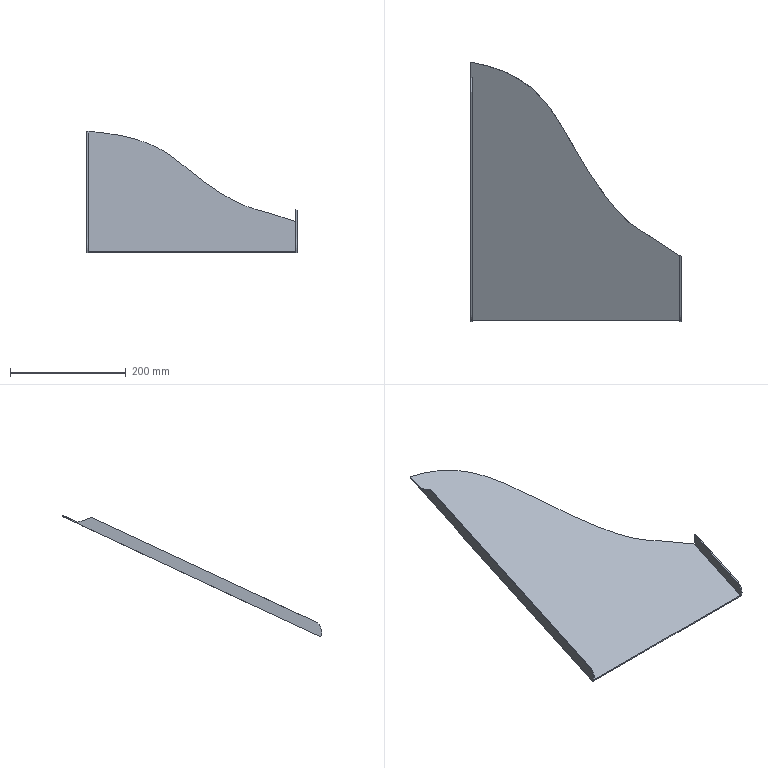Part | NX | features solid 2 | 1 solid | 13 faces | box 363.564 x 448.767 x 210.596 mm | volume 253893 mm3 | plane 10 | cylinder 2 | spline 1 | commonest cylinder face diameters 40 x2
STEP:
#1=CARTESIAN_POINT('',(111.564,-680.,-297.684));
#2=VERTEX_POINT('',#1);
#3=CARTESIAN_POINT('',(-248.,-680.,-297.684));
#4=VERTEX_POINT('',#3);
#5=CARTESIAN_POINT('',(188.564,-680.,-297.684));
#6=DIRECTION('',(1.,0.,0.));
#7=VECTOR('',#6,1000.);
#8=LINE('',#5,#7);
#9=EDGE_CURVE('',#2,#4,#8,.F.);
#10=ORIENTED_EDGE('',*,*,#9,.T.);
#11=CARTESIAN_POINT('',(-248.,-680.,-299.891));
#12=VERTEX_POINT('',#11);
#13=CARTESIAN_POINT('',(-248.,-680.,-430.));
#14=DIRECTION('',(0.,0.,1.));
#15=VECTOR('',#14,1000.);
#16=LINE('',#13,#15);
#17=EDGE_CURVE('',#4,#12,#16,.F.);
#18=ORIENTED_EDGE('',*,*,#17,.T.);
#19=CARTESIAN_POINT('',(111.564,-680.,-299.891));
#20=VERTEX_POINT('',#19);
#21=CARTESIAN_POINT('',(188.564,-680.,-299.891));
#22=DIRECTION('',(1.,0.,0.));
#23=VECTOR('',#22,1000.);
#24=LINE('',#21,#23);
#25=EDGE_CURVE('',#20,#12,#24,.F.);
#26=ORIENTED_EDGE('',*,*,#25,.F.);
#27=CARTESIAN_POINT('',(111.564,-680.,-430.));
#28=DIRECTION('',(0.,0.,1.));
#29=VECTOR('',#28,1000.);
#30=LINE('',#27,#29);
#31=EDGE_CURVE('',#2,#20,#30,.F.);
#32=ORIENTED_EDGE('',*,*,#31,.F.);
#33=EDGE_LOOP('',(#10,#18,#26,#32));
#34=FACE_BOUND('',#33,.T.);
#35=CARTESIAN_POINT('',(188.564,-680.,-430.));
#36=DIRECTION('',(0.,1.,0.));
#37=DIRECTION('',(-1.,0.,0.));
#38=AXIS2_PLACEMENT_3D('',#35,#36,#37);
#39=PLANE('',#38);
#40=ADVANCED_FACE('',(#34),#39,.F.);
#41=CARTESIAN_POINT('',(111.564,-567.729,-245.332));
#42=VERTEX_POINT('',#41);
#43=CARTESIAN_POINT('',(111.564,-570.845,-246.785));
#44=DIRECTION('',(0.,-0.9063,-0.4226));
#45=VECTOR('',#44,1000.);
#46=LINE('',#43,#45);
#47=EDGE_CURVE('',#42,#2,#46,.T.);
#48=ORIENTED_EDGE('',*,*,#47,.F.);
#49=CARTESIAN_POINT('',(-250.,-233.107,-89.295));
#50=VERTEX_POINT('',#49);
#51=CARTESIAN_POINT('',(111.564,-567.729,-245.332));
#52=CARTESIAN_POINT('',(102.698,-561.923,-242.624));
#53=CARTESIAN_POINT('',(89.392,-553.224,-238.568));
#54=CARTESIAN_POINT('',(71.68,-541.588,-233.142));
#55=CARTESIAN_POINT('',(58.379,-532.881,-229.082));
#56=CARTESIAN_POINT('',(44.434,-524.954,-225.385));
#57=CARTESIAN_POINT('',(26.687,-513.356,-219.977));
#58=CARTESIAN_POINT('',(11.101,-499.177,-213.365));
#59=CARTESIAN_POINT('',(-3.01,-483.135,-205.885));
#60=CARTESIAN_POINT('',(-16.196,-466.641,-198.194));
#61=CARTESIAN_POINT('',(-31.486,-445.373,-188.276));
#62=CARTESIAN_POINT('',(-48.725,-419.266,-176.102));
#63=CARTESIAN_POINT('',(-64.763,-392.515,-163.628));
#64=CARTESIAN_POINT('',(-80.04,-365.364,-150.967));
#65=CARTESIAN_POINT('',(-95.517,-338.302,-138.348));
#66=CARTESIAN_POINT('',(-112.708,-312.215,-126.184));
#67=CARTESIAN_POINT('',(-129.476,-292.193,-116.847));
#68=CARTESIAN_POINT('',(-145.224,-277.575,-110.031));
#69=CARTESIAN_POINT('',(-157.985,-267.745,-105.447));
#70=CARTESIAN_POINT('',(-171.635,-259.126,-101.428));
#71=CARTESIAN_POINT('',(-186.187,-251.702,-97.966));
#72=CARTESIAN_POINT('',(-201.622,-245.418,-95.036));
#73=CARTESIAN_POINT('',(-222.673,-238.648,-91.879));
#74=CARTESIAN_POINT('',(-238.985,-235.068,-90.209));
#75=CARTESIAN_POINT('',(-250.,-233.107,-89.295));
#76=B_SPLINE_CURVE_WITH_KNOTS('',3,(#51,#52,#53,#54,#55,#56,#57,#58,#59,#60,#61,#62,#63,#64,#65,#66,#67,#68,#69,#70,#71,#72,#73,#74,#75),.UNSPECIFIED.,.F.,.F.,(4,1,1,1,1,1,1,1,1,1,1,1,1,1,1,1,1,1,1,1,1,1,4),(3.45,3.483,3.499,3.516,3.532,3.549,3.581,3.598,3.614,3.647,3.68,3.713,3.745,3.778,3.811,3.844,3.86,3.877,3.893,3.91,3.926,3.942,3.975),.UNSPECIFIED.);
#77=EDGE_CURVE('',#42,#50,#76,.T.);
#78=ORIENTED_EDGE('',*,*,#77,.T.);
#79=CARTESIAN_POINT('',(-250.,-259.971,-101.822));
#80=VERTEX_POINT('',#79);
#81=CARTESIAN_POINT('',(-250.,-570.845,-246.785));
#82=DIRECTION('',(0.,0.9063,0.4226));
#83=VECTOR('',#82,1000.);
#84=LINE('',#81,#83);
#85=EDGE_CURVE('',#50,#80,#84,.F.);
#86=ORIENTED_EDGE('',*,*,#85,.T.);
#87=CARTESIAN_POINT('',(-248.,-259.971,-101.822));
#88=VERTEX_POINT('',#87);
#89=CARTESIAN_POINT('',(-800.,-259.971,-101.822));
#90=DIRECTION('',(1.,0.,0.));
#91=VECTOR('',#90,1000.);
#92=LINE('',#89,#91);
#93=EDGE_CURVE('',#88,#80,#92,.F.);
#94=ORIENTED_EDGE('',*,*,#93,.F.);
#95=CARTESIAN_POINT('',(-248.,-570.845,-246.785));
#96=DIRECTION('',(0.,-0.9063,-0.4226));
#97=VECTOR('',#96,1000.);
#98=LINE('',#95,#97);
#99=EDGE_CURVE('',#88,#4,#98,.T.);
#100=ORIENTED_EDGE('',*,*,#99,.T.);
#101=ORIENTED_EDGE('',*,*,#9,.F.);
#102=EDGE_LOOP('',(#48,#78,#86,#94,#100,#101));
#103=FACE_BOUND('',#102,.T.);
#104=CARTESIAN_POINT('',(-800.,-570.845,-246.785));
#105=DIRECTION('',(0.,-0.4226,0.9063));
#106=DIRECTION('',(0.,-0.9063,-0.4226));
#107=AXIS2_PLACEMENT_3D('',#104,#105,#106);
#108=PLANE('',#107);
#109=ADVANCED_FACE('',(#103),#108,.T.);
#110=ORIENTED_EDGE('',*,*,#77,.F.);
#111=CARTESIAN_POINT('',(111.564,-567.729,-225.471));
#112=VERTEX_POINT('',#111);
#113=CARTESIAN_POINT('',(111.564,-567.729,-267.464));
#114=DIRECTION('',(0.,0.,1.));
#115=VECTOR('',#114,1000.);
#116=LINE('',#113,#115);
#117=EDGE_CURVE('',#42,#112,#116,.T.);
#118=ORIENTED_EDGE('',*,*,#117,.T.);
#119=CARTESIAN_POINT('',(113.564,-569.039,-226.082));
#120=VERTEX_POINT('',#119);
#121=CARTESIAN_POINT('',(111.564,-567.729,-225.471));
#122=CARTESIAN_POINT('',(112.231,-568.166,-225.674));
#123=CARTESIAN_POINT('',(112.898,-568.602,-225.878));
#124=CARTESIAN_POINT('',(113.564,-569.039,-226.082));
#125=B_SPLINE_CURVE_WITH_KNOTS('',3,(#121,#122,#123,#124),.UNSPECIFIED.,.F.,.F.,(4,4),(-0.1295,-0.1271),.UNSPECIFIED.);
#126=EDGE_CURVE('',#112,#120,#125,.T.);
#127=ORIENTED_EDGE('',*,*,#126,.T.);
#128=CARTESIAN_POINT('',(113.564,-569.039,-248.149));
#129=VERTEX_POINT('',#128);
#130=CARTESIAN_POINT('',(113.564,-569.039,-269.178));
#131=DIRECTION('',(0.,0.,1.));
#132=VECTOR('',#131,1000.);
#133=LINE('',#130,#132);
#134=EDGE_CURVE('',#120,#129,#133,.F.);
#135=ORIENTED_EDGE('',*,*,#134,.T.);
#136=CARTESIAN_POINT('',(-250.,-233.107,-91.502));
#137=VERTEX_POINT('',#136);
#138=CARTESIAN_POINT('',(113.564,-569.039,-248.149));
#139=CARTESIAN_POINT('',(104.432,-563.058,-245.36));
#140=CARTESIAN_POINT('',(90.729,-554.091,-241.179));
#141=CARTESIAN_POINT('',(72.473,-542.122,-235.598));
#142=CARTESIAN_POINT('',(58.806,-533.125,-231.402));
#143=CARTESIAN_POINT('',(44.256,-524.862,-227.549));
#144=CARTESIAN_POINT('',(26.021,-512.876,-221.96));
#145=CARTESIAN_POINT('',(6.706,-495.001,-213.625));
#146=CARTESIAN_POINT('',(-13.173,-470.808,-202.344));
#147=CARTESIAN_POINT('',(-31.517,-445.34,-190.467));
#148=CARTESIAN_POINT('',(-48.868,-419.045,-178.206));
#149=CARTESIAN_POINT('',(-65.147,-391.859,-165.529));
#150=CARTESIAN_POINT('',(-80.74,-364.104,-152.586));
#151=CARTESIAN_POINT('',(-96.57,-336.542,-139.734));
#152=CARTESIAN_POINT('',(-114.056,-310.368,-127.529));
#153=CARTESIAN_POINT('',(-134.465,-286.588,-116.44));
#154=CARTESIAN_POINT('',(-158.481,-266.484,-107.065));
#155=CARTESIAN_POINT('',(-187.039,-250.568,-99.644));
#156=CARTESIAN_POINT('',(-217.596,-239.769,-94.608));
#157=CARTESIAN_POINT('',(-239.141,-235.04,-92.403));
#158=CARTESIAN_POINT('',(-250.,-233.107,-91.502));
#159=B_SPLINE_CURVE_WITH_KNOTS('',3,(#138,#139,#140,#141,#142,#143,#144,#145,#146,#147,#148,#149,#150,#151,#152,#153,#154,#155,#156,#157,#158),.UNSPECIFIED.,.F.,.F.,(4,1,1,1,1,1,1,1,1,1,1,1,1,1,1,1,1,1,4),(0.1269,0.16,0.1765,0.1931,0.2097,0.2262,0.2593,0.2924,0.3255,0.3586,0.3918,0.4249,0.458,0.4911,0.5242,0.5573,0.5904,0.6235,0.6566),.UNSPECIFIED.);
#160=EDGE_CURVE('',#129,#137,#159,.T.);
#161=ORIENTED_EDGE('',*,*,#160,.T.);
#162=CARTESIAN_POINT('',(-250.,-233.107,-89.295));
#163=DIRECTION('',(0.,0.,1.));
#164=VECTOR('',#163,1000.);
#165=LINE('',#162,#164);
#166=EDGE_CURVE('',#50,#137,#165,.F.);
#167=ORIENTED_EDGE('',*,*,#166,.F.);
#168=EDGE_LOOP('',(#110,#118,#127,#135,#161,#167));
#169=FACE_BOUND('',#168,.T.);
#170=CARTESIAN_POINT('',(-250.,-233.107,-249.102));
#171=CARTESIAN_POINT('',(-250.,-233.107,-88.342));
#172=CARTESIAN_POINT('',(-239.339,-235.005,-249.102));
#173=CARTESIAN_POINT('',(-239.339,-235.005,-88.342));
#174=CARTESIAN_POINT('',(-218.009,-239.639,-249.102));
#175=CARTESIAN_POINT('',(-218.009,-239.639,-88.342));
#176=CARTESIAN_POINT('',(-186.633,-250.694,-249.102));
#177=CARTESIAN_POINT('',(-186.633,-250.694,-88.342));
#178=CARTESIAN_POINT('',(-157.179,-267.241,-249.102));
#179=CARTESIAN_POINT('',(-157.179,-267.241,-88.342));
#180=CARTESIAN_POINT('',(-131.588,-289.326,-249.102));
#181=CARTESIAN_POINT('',(-131.588,-289.326,-88.342));
#182=CARTESIAN_POINT('',(-110.563,-315.071,-249.102));
#183=CARTESIAN_POINT('',(-110.563,-315.071,-88.342));
#184=CARTESIAN_POINT('',(-92.999,-342.512,-249.102));
#185=CARTESIAN_POINT('',(-92.999,-342.512,-88.342));
#186=CARTESIAN_POINT('',(-77.274,-370.319,-249.102));
#187=CARTESIAN_POINT('',(-77.274,-370.319,-88.342));
#188=CARTESIAN_POINT('',(-61.764,-397.709,-249.102));
#189=CARTESIAN_POINT('',(-61.764,-397.709,-88.342));
#190=CARTESIAN_POINT('',(-45.456,-424.418,-249.102));
#191=CARTESIAN_POINT('',(-45.456,-424.418,-88.342));
#192=CARTESIAN_POINT('',(-28.01,-450.369,-249.102));
#193=CARTESIAN_POINT('',(-28.01,-450.369,-88.342));
#194=CARTESIAN_POINT('',(-12.615,-471.361,-249.102));
#195=CARTESIAN_POINT('',(-12.615,-471.361,-88.342));
#196=CARTESIAN_POINT('',(0.44,-487.186,-249.102));
#197=CARTESIAN_POINT('',(0.44,-487.186,-88.342));
#198=CARTESIAN_POINT('',(10.739,-498.433,-249.102));
#199=CARTESIAN_POINT('',(10.739,-498.433,-88.342));
#200=CARTESIAN_POINT('',(21.663,-508.711,-249.102));
#201=CARTESIAN_POINT('',(21.663,-508.711,-88.342));
#202=CARTESIAN_POINT('',(33.398,-517.826,-249.102));
#203=CARTESIAN_POINT('',(33.398,-517.826,-88.342));
#204=CARTESIAN_POINT('',(43.982,-524.572,-249.102));
#205=CARTESIAN_POINT('',(43.982,-524.572,-88.342));
#206=CARTESIAN_POINT('',(52.969,-529.82,-249.102));
#207=CARTESIAN_POINT('',(52.969,-529.82,-88.342));
#208=CARTESIAN_POINT('',(59.982,-534.012,-249.102));
#209=CARTESIAN_POINT('',(59.982,-534.012,-88.342));
#210=CARTESIAN_POINT('',(66.879,-538.41,-249.102));
#211=CARTESIAN_POINT('',(66.879,-538.41,-88.342));
#212=CARTESIAN_POINT('',(73.549,-542.833,-249.102));
#213=CARTESIAN_POINT('',(73.549,-542.833,-88.342));
#214=CARTESIAN_POINT('',(80.103,-547.126,-249.102));
#215=CARTESIAN_POINT('',(80.103,-547.126,-88.342));
#216=CARTESIAN_POINT('',(89.03,-552.973,-249.102));
#217=CARTESIAN_POINT('',(89.03,-552.973,-88.342));
#218=CARTESIAN_POINT('',(100.18,-560.274,-249.102));
#219=CARTESIAN_POINT('',(100.18,-560.274,-88.342));
#220=CARTESIAN_POINT('',(109.103,-566.117,-249.102));
#221=CARTESIAN_POINT('',(109.103,-566.117,-88.342));
#222=CARTESIAN_POINT('',(113.564,-569.039,-249.102));
#223=CARTESIAN_POINT('',(113.564,-569.039,-88.342));
#224=B_SPLINE_SURFACE_WITH_KNOTS('',3,1,((#170,#171),(#172,#173),(#174,#175),(#176,#177),(#178,#179),(#180,#181),(#182,#183),(#184,#185),(#186,#187),(#188,#189),(#190,#191),(#192,#193),(#194,#195),(#196,#197),(#198,#199),(#200,#201),(#202,#203),(#204,#205),(#206,#207),(#208,#209),(#210,#211),(#212,#213),(#214,#215),(#216,#217),(#218,#219),(#220,#221),(#222,#223)),.SURF_OF_LINEAR_EXTRUSION.,.F.,.F.,.F.,(4,1,1,1,1,1,1,1,1,1,1,1,1,1,1,1,1,1,1,1,1,1,1,1,4),(2,2),(0.5784,0.6067,0.6351,0.6634,0.6918,0.7201,0.7485,0.7768,0.8052,0.8335,0.8619,0.8903,0.9044,0.9186,0.9328,0.947,0.9611,0.9682,0.9753,0.9824,0.9895,0.9966,1.004,1.018,1.032),(0.,1.),.UNSPECIFIED.);
#225=ADVANCED_FACE('',(#169),#224,.F.);
#226=CARTESIAN_POINT('',(-250.,-680.,-299.891));
#227=VERTEX_POINT('',#226);
#228=CARTESIAN_POINT('',(-250.,-570.,-248.597));
#229=DIRECTION('',(0.,0.9063,0.4226));
#230=VECTOR('',#229,1000.);
#231=LINE('',#228,#230);
#232=EDGE_CURVE('',#137,#227,#231,.F.);
#233=ORIENTED_EDGE('',*,*,#232,.F.);
#234=ORIENTED_EDGE('',*,*,#160,.F.);
#235=CARTESIAN_POINT('',(113.564,-680.,-299.891));
#236=VERTEX_POINT('',#235);
#237=CARTESIAN_POINT('',(113.564,-502.986,-217.348));
#238=DIRECTION('',(0.,-0.9063,-0.4226));
#239=VECTOR('',#238,1000.);
#240=LINE('',#237,#239);
#241=EDGE_CURVE('',#129,#236,#240,.T.);
#242=ORIENTED_EDGE('',*,*,#241,.T.);
#243=CARTESIAN_POINT('',(188.564,-680.,-299.891));
#244=DIRECTION('',(1.,0.,0.));
#245=VECTOR('',#244,1000.);
#246=LINE('',#243,#245);
#247=EDGE_CURVE('',#236,#20,#246,.F.);
#248=ORIENTED_EDGE('',*,*,#247,.T.);
#249=ORIENTED_EDGE('',*,*,#25,.T.);
#250=CARTESIAN_POINT('',(-250.,-680.,-299.891));
#251=DIRECTION('',(1.,0.,0.));
#252=VECTOR('',#251,1000.);
#253=LINE('',#250,#252);
#254=EDGE_CURVE('',#227,#12,#253,.T.);
#255=ORIENTED_EDGE('',*,*,#254,.F.);
#256=EDGE_LOOP('',(#233,#234,#242,#248,#249,#255));
#257=FACE_BOUND('',#256,.T.);
#258=CARTESIAN_POINT('',(-800.,-570.,-248.597));
#259=DIRECTION('',(0.,-0.4226,0.9063));
#260=DIRECTION('',(0.,-0.9063,-0.4226));
#261=AXIS2_PLACEMENT_3D('',#258,#259,#260);
#262=PLANE('',#261);
#263=ADVANCED_FACE('',(#257),#262,.F.);
#264=CARTESIAN_POINT('',(113.564,-670.326,-273.313));
#265=VERTEX_POINT('',#264);
#266=CARTESIAN_POINT('',(113.564,-661.874,-291.439));
#267=DIRECTION('',(1.,0.,0.));
#268=DIRECTION('',(0.,0.,-1.));
#269=AXIS2_PLACEMENT_3D('',#266,#267,#268);
#270=CIRCLE('',#269,20.);
#271=EDGE_CURVE('',#265,#236,#270,.T.);
#272=ORIENTED_EDGE('',*,*,#271,.T.);
#273=ORIENTED_EDGE('',*,*,#241,.F.);
#274=ORIENTED_EDGE('',*,*,#134,.F.);
#275=CARTESIAN_POINT('',(113.564,-564.057,-223.759));
#276=DIRECTION('',(0.,-0.9063,-0.4226));
#277=VECTOR('',#276,1000.);
#278=LINE('',#275,#277);
#279=EDGE_CURVE('',#120,#265,#278,.T.);
#280=ORIENTED_EDGE('',*,*,#279,.T.);
#281=EDGE_LOOP('',(#272,#273,#274,#280));
#282=FACE_BOUND('',#281,.T.);
#283=CARTESIAN_POINT('',(113.564,-503.831,-215.536));
#284=DIRECTION('',(1.,0.,0.));
#285=DIRECTION('',(0.,0.,-1.));
#286=AXIS2_PLACEMENT_3D('',#283,#284,#285);
#287=PLANE('',#286);
#288=ADVANCED_FACE('',(#282),#287,.T.);
#289=ORIENTED_EDGE('',*,*,#126,.F.);
#290=CARTESIAN_POINT('',(111.564,-670.326,-273.313));
#291=VERTEX_POINT('',#290);
#292=CARTESIAN_POINT('',(111.564,-564.057,-223.759));
#293=DIRECTION('',(0.,-0.9063,-0.4226));
#294=VECTOR('',#293,1000.);
#295=LINE('',#292,#294);
#296=EDGE_CURVE('',#112,#291,#295,.T.);
#297=ORIENTED_EDGE('',*,*,#296,.T.);
#298=CARTESIAN_POINT('',(188.564,-670.326,-273.313));
#299=DIRECTION('',(1.,0.,0.));
#300=VECTOR('',#299,1000.);
#301=LINE('',#298,#300);
#302=EDGE_CURVE('',#291,#265,#301,.T.);
#303=ORIENTED_EDGE('',*,*,#302,.T.);
#304=ORIENTED_EDGE('',*,*,#279,.F.);
#305=EDGE_LOOP('',(#289,#297,#303,#304));
#306=FACE_BOUND('',#305,.T.);
#307=CARTESIAN_POINT('',(188.564,-564.057,-223.759));
#308=DIRECTION('',(0.,0.4226,-0.9063));
#309=DIRECTION('',(0.,-0.9063,-0.4226));
#310=AXIS2_PLACEMENT_3D('',#307,#308,#309);
#311=PLANE('',#310);
#312=ADVANCED_FACE('',(#306),#311,.F.);
#313=ORIENTED_EDGE('',*,*,#117,.F.);
#314=ORIENTED_EDGE('',*,*,#47,.T.);
#315=ORIENTED_EDGE('',*,*,#31,.T.);
#316=CARTESIAN_POINT('',(111.564,-661.874,-291.439));
#317=DIRECTION('',(-1.,0.,0.));
#318=DIRECTION('',(0.,0.,1.));
#319=AXIS2_PLACEMENT_3D('',#316,#317,#318);
#320=CIRCLE('',#319,20.);
#321=EDGE_CURVE('',#20,#291,#320,.T.);
#322=ORIENTED_EDGE('',*,*,#321,.T.);
#323=ORIENTED_EDGE('',*,*,#296,.F.);
#324=EDGE_LOOP('',(#313,#314,#315,#322,#323));
#325=FACE_BOUND('',#324,.T.);
#326=CARTESIAN_POINT('',(111.564,-555.605,-241.885));
#327=DIRECTION('',(-1.,0.,0.));
#328=DIRECTION('',(0.,0.,1.));
#329=AXIS2_PLACEMENT_3D('',#326,#327,#328);
#330=PLANE('',#329);
#331=ADVANCED_FACE('',(#325),#330,.T.);
#332=ORIENTED_EDGE('',*,*,#271,.F.);
#333=ORIENTED_EDGE('',*,*,#302,.F.);
#334=ORIENTED_EDGE('',*,*,#321,.F.);
#335=ORIENTED_EDGE('',*,*,#247,.F.);
#336=EDGE_LOOP('',(#332,#333,#334,#335));
#337=FACE_BOUND('',#336,.T.);
#338=CARTESIAN_POINT('',(188.564,-661.874,-291.439));
#339=DIRECTION('',(1.,0.,0.));
#340=DIRECTION('',(0.,0.,-1.));
#341=AXIS2_PLACEMENT_3D('',#338,#339,#340);
#342=CYLINDRICAL_SURFACE('',#341,20.);
#343=ADVANCED_FACE('',(#337),#342,.T.);
#344=ORIENTED_EDGE('',*,*,#232,.T.);
#345=CARTESIAN_POINT('',(-250.,-670.326,-273.313));
#346=VERTEX_POINT('',#345);
#347=CARTESIAN_POINT('',(-250.,-661.874,-291.439));
#348=DIRECTION('',(-1.,0.,0.));
#349=DIRECTION('',(0.,0.,1.));
#350=AXIS2_PLACEMENT_3D('',#347,#348,#349);
#351=CIRCLE('',#350,20.);
#352=EDGE_CURVE('',#227,#346,#351,.T.);
#353=ORIENTED_EDGE('',*,*,#352,.T.);
#354=CARTESIAN_POINT('',(-250.,-283.892,-93.115));
#355=VERTEX_POINT('',#354);
#356=CARTESIAN_POINT('',(-250.,-265.766,-84.663));
#357=DIRECTION('',(0.,-0.9063,-0.4226));
#358=VECTOR('',#357,1000.);
#359=LINE('',#356,#358);
#360=EDGE_CURVE('',#355,#346,#359,.T.);
#361=ORIENTED_EDGE('',*,*,#360,.F.);
#362=CARTESIAN_POINT('',(-250.,-257.313,-102.789));
#363=DIRECTION('',(0.,-0.9397,0.342));
#364=VECTOR('',#363,1000.);
#365=LINE('',#362,#364);
#366=EDGE_CURVE('',#355,#80,#365,.F.);
#367=ORIENTED_EDGE('',*,*,#366,.T.);
#368=ORIENTED_EDGE('',*,*,#85,.F.);
#369=ORIENTED_EDGE('',*,*,#166,.T.);
#370=EDGE_LOOP('',(#344,#353,#361,#367,#368,#369));
#371=FACE_BOUND('',#370,.T.);
#372=CARTESIAN_POINT('',(-250.,-560.,-105.));
#373=DIRECTION('',(1.,0.,0.));
#374=DIRECTION('',(0.,0.,-1.));
#375=AXIS2_PLACEMENT_3D('',#372,#373,#374);
#376=PLANE('',#375);
#377=ADVANCED_FACE('',(#371),#376,.F.);
#378=CARTESIAN_POINT('',(-248.,-283.892,-93.115));
#379=VERTEX_POINT('',#378);
#380=CARTESIAN_POINT('',(-248.,-257.313,-102.789));
#381=DIRECTION('',(0.,0.9397,-0.342));
#382=VECTOR('',#381,1000.);
#383=LINE('',#380,#382);
#384=EDGE_CURVE('',#88,#379,#383,.F.);
#385=ORIENTED_EDGE('',*,*,#384,.F.);
#386=ORIENTED_EDGE('',*,*,#93,.T.);
#387=ORIENTED_EDGE('',*,*,#366,.F.);
#388=CARTESIAN_POINT('',(-250.,-283.892,-93.115));
#389=DIRECTION('',(1.,0.,0.));
#390=VECTOR('',#389,1000.);
#391=LINE('',#388,#390);
#392=EDGE_CURVE('',#379,#355,#391,.F.);
#393=ORIENTED_EDGE('',*,*,#392,.F.);
#394=EDGE_LOOP('',(#385,#386,#387,#393));
#395=FACE_BOUND('',#394,.T.);
#396=CARTESIAN_POINT('',(-250.,-257.313,-102.789));
#397=DIRECTION('',(0.,-0.342,-0.9397));
#398=DIRECTION('',(0.,0.9397,-0.342));
#399=AXIS2_PLACEMENT_3D('',#396,#397,#398);
#400=PLANE('',#399);
#401=ADVANCED_FACE('',(#395),#400,.F.);
#402=ORIENTED_EDGE('',*,*,#352,.F.);
#403=ORIENTED_EDGE('',*,*,#254,.T.);
#404=CARTESIAN_POINT('',(-248.,-670.326,-273.313));
#405=VERTEX_POINT('',#404);
#406=CARTESIAN_POINT('',(-248.,-661.874,-291.439));
#407=DIRECTION('',(-1.,0.,0.));
#408=DIRECTION('',(0.,0.,1.));
#409=AXIS2_PLACEMENT_3D('',#406,#407,#408);
#410=CIRCLE('',#409,20.);
#411=EDGE_CURVE('',#405,#12,#410,.F.);
#412=ORIENTED_EDGE('',*,*,#411,.F.);
#413=CARTESIAN_POINT('',(-250.,-670.326,-273.313));
#414=DIRECTION('',(1.,0.,0.));
#415=VECTOR('',#414,1000.);
#416=LINE('',#413,#415);
#417=EDGE_CURVE('',#346,#405,#416,.T.);
#418=ORIENTED_EDGE('',*,*,#417,.F.);
#419=EDGE_LOOP('',(#402,#403,#412,#418));
#420=FACE_BOUND('',#419,.T.);
#421=CARTESIAN_POINT('',(-250.,-661.874,-291.439));
#422=DIRECTION('',(-1.,0.,0.));
#423=DIRECTION('',(0.,0.,1.));
#424=AXIS2_PLACEMENT_3D('',#421,#422,#423);
#425=CYLINDRICAL_SURFACE('',#424,20.);
#426=ADVANCED_FACE('',(#420),#425,.T.);
#427=ORIENTED_EDGE('',*,*,#17,.F.);
#428=ORIENTED_EDGE('',*,*,#99,.F.);
#429=ORIENTED_EDGE('',*,*,#384,.T.);
#430=CARTESIAN_POINT('',(-248.,-265.766,-84.663));
#431=DIRECTION('',(0.,-0.9063,-0.4226));
#432=VECTOR('',#431,1000.);
#433=LINE('',#430,#432);
#434=EDGE_CURVE('',#379,#405,#433,.T.);
#435=ORIENTED_EDGE('',*,*,#434,.T.);
#436=ORIENTED_EDGE('',*,*,#411,.T.);
#437=EDGE_LOOP('',(#427,#428,#429,#435,#436));
#438=FACE_BOUND('',#437,.T.);
#439=CARTESIAN_POINT('',(-248.,-257.313,-102.789));
#440=DIRECTION('',(-1.,0.,0.));
#441=DIRECTION('',(0.,0.,1.));
#442=AXIS2_PLACEMENT_3D('',#439,#440,#441);
#443=PLANE('',#442);
#444=ADVANCED_FACE('',(#438),#443,.F.);
#445=ORIENTED_EDGE('',*,*,#434,.F.);
#446=ORIENTED_EDGE('',*,*,#392,.T.);
#447=ORIENTED_EDGE('',*,*,#360,.T.);
#448=ORIENTED_EDGE('',*,*,#417,.T.);
#449=EDGE_LOOP('',(#445,#446,#447,#448));
#450=FACE_BOUND('',#449,.T.);
#451=CARTESIAN_POINT('',(-250.,-265.766,-84.663));
#452=DIRECTION('',(0.,0.4226,-0.9063));
#453=DIRECTION('',(0.,-0.9063,-0.4226));
#454=AXIS2_PLACEMENT_3D('',#451,#452,#453);
#455=PLANE('',#454);
#456=ADVANCED_FACE('',(#450),#455,.F.);
#457=CLOSED_SHELL('',(#40,#109,#225,#263,#288,#312,#331,#343,#377,#401,#426,#444,#456));
#458=MANIFOLD_SOLID_BREP('',#457);
#459=(LENGTH_UNIT()NAMED_UNIT(*)SI_UNIT(.MILLI.,.METRE.));
#460=UNCERTAINTY_MEASURE_WITH_UNIT(LENGTH_MEASURE(0.0508),#459,'','');
#461=(NAMED_UNIT(*)PLANE_ANGLE_UNIT()SI_UNIT($,.RADIAN.));
#462=(NAMED_UNIT(*)SI_UNIT($,.STERADIAN.)SOLID_ANGLE_UNIT());
#463=(GEOMETRIC_REPRESENTATION_CONTEXT(3)GLOBAL_UNCERTAINTY_ASSIGNED_CONTEXT((#460))GLOBAL_UNIT_ASSIGNED_CONTEXT((#459,#461,#462))REPRESENTATION_CONTEXT('',''));
#464=ADVANCED_BREP_SHAPE_REPRESENTATION('',(#458),#463);